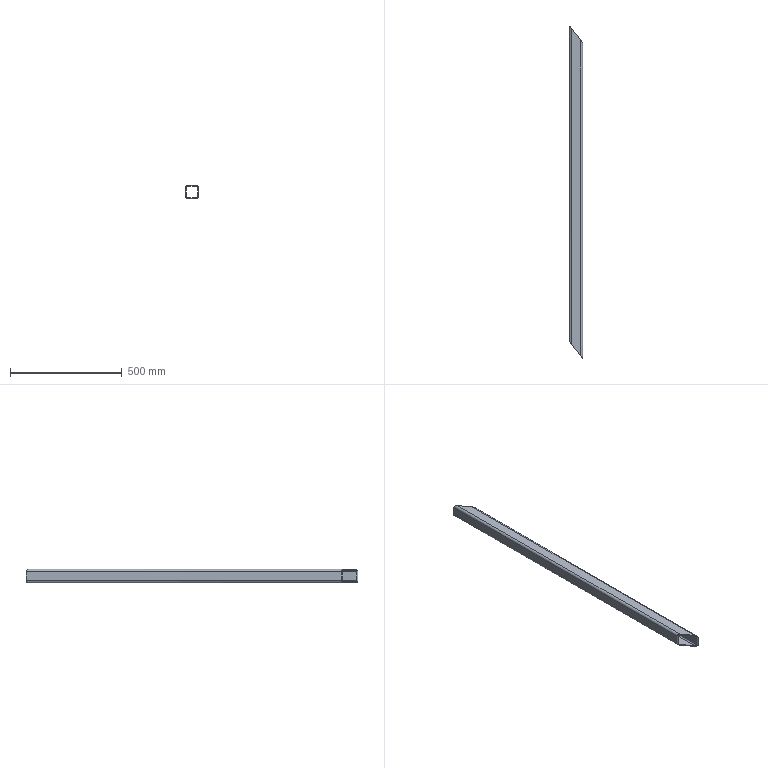Part | SolidWorks | features Extrusion 1, ICE 1 | 1 solid | 18 faces | box 60 x 1484 x 60 mm | volume 1185056 mm3 | plane 10 | cylinder 8 | commonest cylinder face diameters 12 x4 20 x4
STEP:
#1=CARTESIAN_POINT('',(-26.,70.025,-20.));
#2=VERTEX_POINT('',#1);
#3=CARTESIAN_POINT('',(-26.,70.025,20.));
#4=VERTEX_POINT('',#3);
#5=CARTESIAN_POINT('',(-26.,70.025,20.));
#6=DIRECTION('',(0.,0.,1.));
#7=VECTOR('',#6,1000.);
#8=LINE('',#5,#7);
#9=EDGE_CURVE('',#2,#4,#8,.T.);
#10=ORIENTED_EDGE('',*,*,#9,.F.);
#11=CARTESIAN_POINT('',(-26.,1479.025,-20.));
#12=VERTEX_POINT('',#11);
#13=CARTESIAN_POINT('',(-26.,2000.,-20.));
#14=DIRECTION('',(0.,-1.,0.));
#15=VECTOR('',#14,1000.);
#16=LINE('',#13,#15);
#17=EDGE_CURVE('',#12,#2,#16,.T.);
#18=ORIENTED_EDGE('',*,*,#17,.F.);
#19=CARTESIAN_POINT('',(-26.,1479.025,20.));
#20=VERTEX_POINT('',#19);
#21=CARTESIAN_POINT('',(-26.,1479.025,20.));
#22=DIRECTION('',(0.,0.,-1.));
#23=VECTOR('',#22,1000.);
#24=LINE('',#21,#23);
#25=EDGE_CURVE('',#20,#12,#24,.T.);
#26=ORIENTED_EDGE('',*,*,#25,.F.);
#27=CARTESIAN_POINT('',(-26.,2000.,20.));
#28=DIRECTION('',(0.,-1.,0.));
#29=VECTOR('',#28,1000.);
#30=LINE('',#27,#29);
#31=EDGE_CURVE('',#20,#4,#30,.T.);
#32=ORIENTED_EDGE('',*,*,#31,.T.);
#33=EDGE_LOOP('',(#10,#18,#26,#32));
#34=FACE_OUTER_BOUND('',#33,.T.);
#35=CARTESIAN_POINT('',(-26.,2000.,20.));
#36=DIRECTION('',(1.,0.,0.));
#37=DIRECTION('',(0.,0.,-1.));
#38=AXIS2_PLACEMENT_3D('',#35,#36,#37);
#39=PLANE('',#38);
#40=ADVANCED_FACE('',(#34),#39,.T.);
#41=CARTESIAN_POINT('',(-20.,62.523,-26.));
#42=VERTEX_POINT('',#41);
#43=CARTESIAN_POINT('',(-20.,62.523,-26.));
#44=CARTESIAN_POINT('',(-23.515,66.918,-26.));
#45=CARTESIAN_POINT('',(-26.,70.025,-23.515));
#46=CARTESIAN_POINT('',(-26.,70.025,-20.));
#47=(BOUNDED_CURVE()B_SPLINE_CURVE(3,(#43,#44,#45,#46),.UNSPECIFIED.,.F.,.T.)B_SPLINE_CURVE_WITH_KNOTS((4,4),(1.571,3.142),.UNSPECIFIED.)CURVE()GEOMETRIC_REPRESENTATION_ITEM()RATIONAL_B_SPLINE_CURVE((1.,0.8047,0.8047,1.))REPRESENTATION_ITEM(''));
#48=EDGE_CURVE('',#42,#2,#47,.T.);
#49=ORIENTED_EDGE('',*,*,#48,.F.);
#50=CARTESIAN_POINT('',(-20.,1471.523,-26.));
#51=VERTEX_POINT('',#50);
#52=CARTESIAN_POINT('',(-20.,2000.,-26.));
#53=DIRECTION('',(0.,-1.,0.));
#54=VECTOR('',#53,1000.);
#55=LINE('',#52,#54);
#56=EDGE_CURVE('',#51,#42,#55,.T.);
#57=ORIENTED_EDGE('',*,*,#56,.F.);
#58=CARTESIAN_POINT('',(-26.,1479.025,-20.));
#59=CARTESIAN_POINT('',(-26.,1479.025,-23.515));
#60=CARTESIAN_POINT('',(-23.515,1475.918,-26.));
#61=CARTESIAN_POINT('',(-20.,1471.523,-26.));
#62=(BOUNDED_CURVE()B_SPLINE_CURVE(3,(#58,#59,#60,#61),.UNSPECIFIED.,.F.,.F.)B_SPLINE_CURVE_WITH_KNOTS((4,4),(3.142,4.712),.UNSPECIFIED.)CURVE()GEOMETRIC_REPRESENTATION_ITEM()RATIONAL_B_SPLINE_CURVE((1.,0.8047,0.8047,1.))REPRESENTATION_ITEM(''));
#63=EDGE_CURVE('',#12,#51,#62,.T.);
#64=ORIENTED_EDGE('',*,*,#63,.F.);
#65=ORIENTED_EDGE('',*,*,#17,.T.);
#66=EDGE_LOOP('',(#49,#57,#64,#65));
#67=FACE_OUTER_BOUND('',#66,.T.);
#68=CARTESIAN_POINT('',(-20.,2000.,-20.));
#69=DIRECTION('',(0.,-1.,0.));
#70=DIRECTION('',(0.,0.,-1.));
#71=AXIS2_PLACEMENT_3D('',#68,#69,#70);
#72=CYLINDRICAL_SURFACE('',#71,6.);
#73=ADVANCED_FACE('',(#67),#72,.F.);
#74=CARTESIAN_POINT('',(20.,12.505,-26.));
#75=VERTEX_POINT('',#74);
#76=CARTESIAN_POINT('',(-965.035,1244.247,-26.));
#77=DIRECTION('',(-0.6246,0.781,0.));
#78=VECTOR('',#77,1000.);
#79=LINE('',#76,#78);
#80=EDGE_CURVE('',#75,#42,#79,.T.);
#81=ORIENTED_EDGE('',*,*,#80,.F.);
#82=CARTESIAN_POINT('',(20.,1421.505,-26.));
#83=VERTEX_POINT('',#82);
#84=CARTESIAN_POINT('',(20.,2000.,-26.));
#85=DIRECTION('',(0.,-1.,0.));
#86=VECTOR('',#85,1000.);
#87=LINE('',#84,#86);
#88=EDGE_CURVE('',#83,#75,#87,.T.);
#89=ORIENTED_EDGE('',*,*,#88,.F.);
#90=CARTESIAN_POINT('',(-277.773,1793.856,-26.));
#91=DIRECTION('',(0.6246,-0.781,0.));
#92=VECTOR('',#91,1000.);
#93=LINE('',#90,#92);
#94=EDGE_CURVE('',#51,#83,#93,.T.);
#95=ORIENTED_EDGE('',*,*,#94,.F.);
#96=ORIENTED_EDGE('',*,*,#56,.T.);
#97=EDGE_LOOP('',(#81,#89,#95,#96));
#98=FACE_OUTER_BOUND('',#97,.T.);
#99=CARTESIAN_POINT('',(-20.,2000.,-26.));
#100=DIRECTION('',(0.,0.,1.));
#101=DIRECTION('',(1.,0.,0.));
#102=AXIS2_PLACEMENT_3D('',#99,#100,#101);
#103=PLANE('',#102);
#104=ADVANCED_FACE('',(#98),#103,.T.);
#105=CARTESIAN_POINT('',(26.,5.002,-20.));
#106=VERTEX_POINT('',#105);
#107=CARTESIAN_POINT('',(26.,5.002,-20.));
#108=CARTESIAN_POINT('',(26.,5.002,-23.515));
#109=CARTESIAN_POINT('',(23.515,8.11,-26.));
#110=CARTESIAN_POINT('',(20.,12.505,-26.));
#111=(BOUNDED_CURVE()B_SPLINE_CURVE(3,(#107,#108,#109,#110),.UNSPECIFIED.,.F.,.F.)B_SPLINE_CURVE_WITH_KNOTS((4,4),(0.,1.571),.UNSPECIFIED.)CURVE()GEOMETRIC_REPRESENTATION_ITEM()RATIONAL_B_SPLINE_CURVE((1.,0.8047,0.8047,1.))REPRESENTATION_ITEM(''));
#112=EDGE_CURVE('',#106,#75,#111,.T.);
#113=ORIENTED_EDGE('',*,*,#112,.F.);
#114=CARTESIAN_POINT('',(26.,1414.002,-20.));
#115=VERTEX_POINT('',#114);
#116=CARTESIAN_POINT('',(26.,2000.,-20.));
#117=DIRECTION('',(0.,-1.,0.));
#118=VECTOR('',#117,1000.);
#119=LINE('',#116,#118);
#120=EDGE_CURVE('',#115,#106,#119,.T.);
#121=ORIENTED_EDGE('',*,*,#120,.F.);
#122=CARTESIAN_POINT('',(20.,1421.505,-26.));
#123=CARTESIAN_POINT('',(23.515,1417.11,-26.));
#124=CARTESIAN_POINT('',(26.,1414.002,-23.515));
#125=CARTESIAN_POINT('',(26.,1414.002,-20.));
#126=(BOUNDED_CURVE()B_SPLINE_CURVE(3,(#122,#123,#124,#125),.UNSPECIFIED.,.F.,.T.)B_SPLINE_CURVE_WITH_KNOTS((4,4),(4.712,6.283),.UNSPECIFIED.)CURVE()GEOMETRIC_REPRESENTATION_ITEM()RATIONAL_B_SPLINE_CURVE((1.,0.8047,0.8047,1.))REPRESENTATION_ITEM(''));
#127=EDGE_CURVE('',#83,#115,#126,.T.);
#128=ORIENTED_EDGE('',*,*,#127,.F.);
#129=ORIENTED_EDGE('',*,*,#88,.T.);
#130=EDGE_LOOP('',(#113,#121,#128,#129));
#131=FACE_OUTER_BOUND('',#130,.T.);
#132=CARTESIAN_POINT('',(20.,2000.,-20.));
#133=DIRECTION('',(0.,-1.,0.));
#134=DIRECTION('',(0.,0.,-1.));
#135=AXIS2_PLACEMENT_3D('',#132,#133,#134);
#136=CYLINDRICAL_SURFACE('',#135,6.);
#137=ADVANCED_FACE('',(#131),#136,.F.);
#138=CARTESIAN_POINT('',(26.,5.002,20.));
#139=VERTEX_POINT('',#138);
#140=CARTESIAN_POINT('',(26.,5.002,20.));
#141=DIRECTION('',(0.,0.,-1.));
#142=VECTOR('',#141,1000.);
#143=LINE('',#140,#142);
#144=EDGE_CURVE('',#139,#106,#143,.T.);
#145=ORIENTED_EDGE('',*,*,#144,.F.);
#146=CARTESIAN_POINT('',(26.,1414.002,20.));
#147=VERTEX_POINT('',#146);
#148=CARTESIAN_POINT('',(26.,2000.,20.));
#149=DIRECTION('',(0.,-1.,0.));
#150=VECTOR('',#149,1000.);
#151=LINE('',#148,#150);
#152=EDGE_CURVE('',#147,#139,#151,.T.);
#153=ORIENTED_EDGE('',*,*,#152,.F.);
#154=CARTESIAN_POINT('',(26.,1414.002,20.));
#155=DIRECTION('',(0.,0.,1.));
#156=VECTOR('',#155,1000.);
#157=LINE('',#154,#156);
#158=EDGE_CURVE('',#115,#147,#157,.T.);
#159=ORIENTED_EDGE('',*,*,#158,.F.);
#160=ORIENTED_EDGE('',*,*,#120,.T.);
#161=EDGE_LOOP('',(#145,#153,#159,#160));
#162=FACE_OUTER_BOUND('',#161,.T.);
#163=CARTESIAN_POINT('',(26.,2000.,20.));
#164=DIRECTION('',(-1.,0.,0.));
#165=DIRECTION('',(0.,0.,1.));
#166=AXIS2_PLACEMENT_3D('',#163,#164,#165);
#167=PLANE('',#166);
#168=ADVANCED_FACE('',(#162),#167,.T.);
#169=CARTESIAN_POINT('',(20.,12.505,26.));
#170=VERTEX_POINT('',#169);
#171=CARTESIAN_POINT('',(20.,12.505,26.));
#172=CARTESIAN_POINT('',(23.515,8.11,26.));
#173=CARTESIAN_POINT('',(26.,5.002,23.515));
#174=CARTESIAN_POINT('',(26.,5.002,20.));
#175=(BOUNDED_CURVE()B_SPLINE_CURVE(3,(#171,#172,#173,#174),.UNSPECIFIED.,.F.,.F.)B_SPLINE_CURVE_WITH_KNOTS((4,4),(4.712,6.283),.UNSPECIFIED.)CURVE()GEOMETRIC_REPRESENTATION_ITEM()RATIONAL_B_SPLINE_CURVE((1.,0.8047,0.8047,1.))REPRESENTATION_ITEM(''));
#176=EDGE_CURVE('',#170,#139,#175,.T.);
#177=ORIENTED_EDGE('',*,*,#176,.F.);
#178=CARTESIAN_POINT('',(20.,1421.505,26.));
#179=VERTEX_POINT('',#178);
#180=CARTESIAN_POINT('',(20.,2000.,26.));
#181=DIRECTION('',(0.,-1.,0.));
#182=VECTOR('',#181,1000.);
#183=LINE('',#180,#182);
#184=EDGE_CURVE('',#179,#170,#183,.T.);
#185=ORIENTED_EDGE('',*,*,#184,.F.);
#186=CARTESIAN_POINT('',(26.,1414.002,20.));
#187=CARTESIAN_POINT('',(26.,1414.002,23.515));
#188=CARTESIAN_POINT('',(23.515,1417.11,26.));
#189=CARTESIAN_POINT('',(20.,1421.505,26.));
#190=(BOUNDED_CURVE()B_SPLINE_CURVE(3,(#186,#187,#188,#189),.UNSPECIFIED.,.F.,.T.)B_SPLINE_CURVE_WITH_KNOTS((4,4),(0.,1.571),.UNSPECIFIED.)CURVE()GEOMETRIC_REPRESENTATION_ITEM()RATIONAL_B_SPLINE_CURVE((1.,0.8047,0.8047,1.))REPRESENTATION_ITEM(''));
#191=EDGE_CURVE('',#147,#179,#190,.T.);
#192=ORIENTED_EDGE('',*,*,#191,.F.);
#193=ORIENTED_EDGE('',*,*,#152,.T.);
#194=EDGE_LOOP('',(#177,#185,#192,#193));
#195=FACE_OUTER_BOUND('',#194,.T.);
#196=CARTESIAN_POINT('',(20.,2000.,20.));
#197=DIRECTION('',(0.,-1.,0.));
#198=DIRECTION('',(0.,0.,-1.));
#199=AXIS2_PLACEMENT_3D('',#196,#197,#198);
#200=CYLINDRICAL_SURFACE('',#199,6.);
#201=ADVANCED_FACE('',(#195),#200,.F.);
#202=CARTESIAN_POINT('',(-20.,62.523,26.));
#203=VERTEX_POINT('',#202);
#204=CARTESIAN_POINT('',(-965.035,1244.247,26.));
#205=DIRECTION('',(0.6246,-0.781,0.));
#206=VECTOR('',#205,1000.);
#207=LINE('',#204,#206);
#208=EDGE_CURVE('',#203,#170,#207,.T.);
#209=ORIENTED_EDGE('',*,*,#208,.F.);
#210=CARTESIAN_POINT('',(-20.,1471.523,26.));
#211=VERTEX_POINT('',#210);
#212=CARTESIAN_POINT('',(-20.,2000.,26.));
#213=DIRECTION('',(0.,-1.,0.));
#214=VECTOR('',#213,1000.);
#215=LINE('',#212,#214);
#216=EDGE_CURVE('',#211,#203,#215,.T.);
#217=ORIENTED_EDGE('',*,*,#216,.F.);
#218=CARTESIAN_POINT('',(-277.773,1793.856,26.));
#219=DIRECTION('',(-0.6246,0.781,0.));
#220=VECTOR('',#219,1000.);
#221=LINE('',#218,#220);
#222=EDGE_CURVE('',#179,#211,#221,.T.);
#223=ORIENTED_EDGE('',*,*,#222,.F.);
#224=ORIENTED_EDGE('',*,*,#184,.T.);
#225=EDGE_LOOP('',(#209,#217,#223,#224));
#226=FACE_OUTER_BOUND('',#225,.T.);
#227=CARTESIAN_POINT('',(-20.,2000.,26.));
#228=DIRECTION('',(0.,0.,-1.));
#229=DIRECTION('',(-1.,0.,0.));
#230=AXIS2_PLACEMENT_3D('',#227,#228,#229);
#231=PLANE('',#230);
#232=ADVANCED_FACE('',(#226),#231,.T.);
#233=CARTESIAN_POINT('',(-26.,70.025,20.));
#234=CARTESIAN_POINT('',(-26.,70.025,23.515));
#235=CARTESIAN_POINT('',(-23.515,66.918,26.));
#236=CARTESIAN_POINT('',(-20.,62.523,26.));
#237=(BOUNDED_CURVE()B_SPLINE_CURVE(3,(#233,#234,#235,#236),.UNSPECIFIED.,.F.,.F.)B_SPLINE_CURVE_WITH_KNOTS((4,4),(3.142,4.712),.UNSPECIFIED.)CURVE()GEOMETRIC_REPRESENTATION_ITEM()RATIONAL_B_SPLINE_CURVE((1.,0.8047,0.8047,1.))REPRESENTATION_ITEM(''));
#238=EDGE_CURVE('',#4,#203,#237,.T.);
#239=ORIENTED_EDGE('',*,*,#238,.F.);
#240=ORIENTED_EDGE('',*,*,#31,.F.);
#241=CARTESIAN_POINT('',(-20.,1471.523,26.));
#242=CARTESIAN_POINT('',(-23.515,1475.918,26.));
#243=CARTESIAN_POINT('',(-26.,1479.025,23.515));
#244=CARTESIAN_POINT('',(-26.,1479.025,20.));
#245=(BOUNDED_CURVE()B_SPLINE_CURVE(3,(#241,#242,#243,#244),.UNSPECIFIED.,.F.,.T.)B_SPLINE_CURVE_WITH_KNOTS((4,4),(1.571,3.142),.UNSPECIFIED.)CURVE()GEOMETRIC_REPRESENTATION_ITEM()RATIONAL_B_SPLINE_CURVE((1.,0.8047,0.8047,1.))REPRESENTATION_ITEM(''));
#246=EDGE_CURVE('',#211,#20,#245,.T.);
#247=ORIENTED_EDGE('',*,*,#246,.F.);
#248=ORIENTED_EDGE('',*,*,#216,.T.);
#249=EDGE_LOOP('',(#239,#240,#247,#248));
#250=FACE_OUTER_BOUND('',#249,.T.);
#251=CARTESIAN_POINT('',(-20.,2000.,20.));
#252=DIRECTION('',(0.,-1.,0.));
#253=DIRECTION('',(0.,0.,-1.));
#254=AXIS2_PLACEMENT_3D('',#251,#252,#253);
#255=CYLINDRICAL_SURFACE('',#254,6.);
#256=ADVANCED_FACE('',(#250),#255,.F.);
#257=ORIENTED_EDGE('',*,*,#246,.T.);
#258=ORIENTED_EDGE('',*,*,#25,.T.);
#259=ORIENTED_EDGE('',*,*,#63,.T.);
#260=ORIENTED_EDGE('',*,*,#94,.T.);
#261=ORIENTED_EDGE('',*,*,#127,.T.);
#262=ORIENTED_EDGE('',*,*,#158,.T.);
#263=ORIENTED_EDGE('',*,*,#191,.T.);
#264=ORIENTED_EDGE('',*,*,#222,.T.);
#265=EDGE_LOOP('',(#257,#258,#259,#260,#261,#262,#263,#264));
#266=FACE_BOUND('',#265,.T.);
#267=CARTESIAN_POINT('',(-20.,1471.523,-30.));
#268=VERTEX_POINT('',#267);
#269=CARTESIAN_POINT('',(20.,1421.505,-30.));
#270=VERTEX_POINT('',#269);
#271=CARTESIAN_POINT('',(-30.,1484.027,-30.));
#272=DIRECTION('',(0.6246,-0.781,0.));
#273=VECTOR('',#272,1000.);
#274=LINE('',#271,#273);
#275=EDGE_CURVE('',#268,#270,#274,.T.);
#276=ORIENTED_EDGE('',*,*,#275,.F.);
#277=CARTESIAN_POINT('',(-30.,1484.027,-20.));
#278=VERTEX_POINT('',#277);
#279=CARTESIAN_POINT('',(-30.,1484.027,-20.));
#280=CARTESIAN_POINT('',(-30.,1484.027,-25.858));
#281=CARTESIAN_POINT('',(-25.858,1478.848,-30.));
#282=CARTESIAN_POINT('',(-20.,1471.523,-30.));
#283=(BOUNDED_CURVE()B_SPLINE_CURVE(3,(#279,#280,#281,#282),.UNSPECIFIED.,.F.,.F.)B_SPLINE_CURVE_WITH_KNOTS((4,4),(3.142,4.712),.UNSPECIFIED.)CURVE()GEOMETRIC_REPRESENTATION_ITEM()RATIONAL_B_SPLINE_CURVE((1.,0.8047,0.8047,1.))REPRESENTATION_ITEM(''));
#284=EDGE_CURVE('',#278,#268,#283,.T.);
#285=ORIENTED_EDGE('',*,*,#284,.F.);
#286=CARTESIAN_POINT('',(-30.,1484.027,20.));
#287=VERTEX_POINT('',#286);
#288=CARTESIAN_POINT('',(-30.,1484.027,-30.));
#289=DIRECTION('',(0.,0.,1.));
#290=VECTOR('',#289,1000.);
#291=LINE('',#288,#290);
#292=EDGE_CURVE('',#278,#287,#291,.T.);
#293=ORIENTED_EDGE('',*,*,#292,.T.);
#294=CARTESIAN_POINT('',(-20.,1471.523,30.));
#295=VERTEX_POINT('',#294);
#296=CARTESIAN_POINT('',(-20.,1471.523,30.));
#297=CARTESIAN_POINT('',(-25.858,1478.848,30.));
#298=CARTESIAN_POINT('',(-30.,1484.027,25.858));
#299=CARTESIAN_POINT('',(-30.,1484.027,20.));
#300=(BOUNDED_CURVE()B_SPLINE_CURVE(3,(#296,#297,#298,#299),.UNSPECIFIED.,.F.,.T.)B_SPLINE_CURVE_WITH_KNOTS((4,4),(1.571,3.142),.UNSPECIFIED.)CURVE()GEOMETRIC_REPRESENTATION_ITEM()RATIONAL_B_SPLINE_CURVE((1.,0.8047,0.8047,1.))REPRESENTATION_ITEM(''));
#301=EDGE_CURVE('',#295,#287,#300,.T.);
#302=ORIENTED_EDGE('',*,*,#301,.F.);
#303=CARTESIAN_POINT('',(20.,1421.505,30.));
#304=VERTEX_POINT('',#303);
#305=CARTESIAN_POINT('',(-277.773,1793.856,30.));
#306=DIRECTION('',(-0.6246,0.781,0.));
#307=VECTOR('',#306,1000.);
#308=LINE('',#305,#307);
#309=EDGE_CURVE('',#304,#295,#308,.T.);
#310=ORIENTED_EDGE('',*,*,#309,.F.);
#311=CARTESIAN_POINT('',(30.,1409.,20.));
#312=VERTEX_POINT('',#311);
#313=CARTESIAN_POINT('',(30.,1409.,20.));
#314=CARTESIAN_POINT('',(30.,1409.,25.858));
#315=CARTESIAN_POINT('',(25.858,1414.18,30.));
#316=CARTESIAN_POINT('',(20.,1421.505,30.));
#317=(BOUNDED_CURVE()B_SPLINE_CURVE(3,(#313,#314,#315,#316),.UNSPECIFIED.,.F.,.F.)B_SPLINE_CURVE_WITH_KNOTS((4,4),(0.,1.571),.UNSPECIFIED.)CURVE()GEOMETRIC_REPRESENTATION_ITEM()RATIONAL_B_SPLINE_CURVE((1.,0.8047,0.8047,1.))REPRESENTATION_ITEM(''));
#318=EDGE_CURVE('',#312,#304,#317,.T.);
#319=ORIENTED_EDGE('',*,*,#318,.F.);
#320=CARTESIAN_POINT('',(30.,1409.,-20.));
#321=VERTEX_POINT('',#320);
#322=CARTESIAN_POINT('',(30.,1409.,-30.));
#323=DIRECTION('',(0.,0.,1.));
#324=VECTOR('',#323,1000.);
#325=LINE('',#322,#324);
#326=EDGE_CURVE('',#321,#312,#325,.T.);
#327=ORIENTED_EDGE('',*,*,#326,.F.);
#328=CARTESIAN_POINT('',(20.,1421.505,-30.));
#329=CARTESIAN_POINT('',(25.858,1414.18,-30.));
#330=CARTESIAN_POINT('',(30.,1409.,-25.858));
#331=CARTESIAN_POINT('',(30.,1409.,-20.));
#332=(BOUNDED_CURVE()B_SPLINE_CURVE(3,(#328,#329,#330,#331),.UNSPECIFIED.,.F.,.F.)B_SPLINE_CURVE_WITH_KNOTS((4,4),(4.712,6.283),.UNSPECIFIED.)CURVE()GEOMETRIC_REPRESENTATION_ITEM()RATIONAL_B_SPLINE_CURVE((1.,0.8047,0.8047,1.))REPRESENTATION_ITEM(''));
#333=EDGE_CURVE('',#270,#321,#332,.T.);
#334=ORIENTED_EDGE('',*,*,#333,.F.);
#335=EDGE_LOOP('',(#276,#285,#293,#302,#310,#319,#327,#334));
#336=FACE_OUTER_BOUND('',#335,.T.);
#337=CARTESIAN_POINT('',(-30.,1484.027,-30.));
#338=DIRECTION('',(-0.781,-0.6246,0.));
#339=DIRECTION('',(0.6246,-0.781,0.));
#340=AXIS2_PLACEMENT_3D('',#337,#338,#339);
#341=PLANE('',#340);
#342=ADVANCED_FACE('',(#266,#336),#341,.F.);
#343=ORIENTED_EDGE('',*,*,#238,.T.);
#344=ORIENTED_EDGE('',*,*,#208,.T.);
#345=ORIENTED_EDGE('',*,*,#176,.T.);
#346=ORIENTED_EDGE('',*,*,#144,.T.);
#347=ORIENTED_EDGE('',*,*,#112,.T.);
#348=ORIENTED_EDGE('',*,*,#80,.T.);
#349=ORIENTED_EDGE('',*,*,#48,.T.);
#350=ORIENTED_EDGE('',*,*,#9,.T.);
#351=EDGE_LOOP('',(#343,#344,#345,#346,#347,#348,#349,#350));
#352=FACE_BOUND('',#351,.T.);
#353=CARTESIAN_POINT('',(30.,0.,20.));
#354=VERTEX_POINT('',#353);
#355=CARTESIAN_POINT('',(30.,0.,-20.));
#356=VERTEX_POINT('',#355);
#357=CARTESIAN_POINT('',(30.,0.,20.));
#358=DIRECTION('',(0.,0.,-1.));
#359=VECTOR('',#358,1000.);
#360=LINE('',#357,#359);
#361=EDGE_CURVE('',#354,#356,#360,.T.);
#362=ORIENTED_EDGE('',*,*,#361,.F.);
#363=CARTESIAN_POINT('',(20.,12.505,30.));
#364=VERTEX_POINT('',#363);
#365=CARTESIAN_POINT('',(20.,12.505,30.));
#366=CARTESIAN_POINT('',(25.858,5.18,30.));
#367=CARTESIAN_POINT('',(30.,0.,25.858));
#368=CARTESIAN_POINT('',(30.,0.,20.));
#369=(BOUNDED_CURVE()B_SPLINE_CURVE(3,(#365,#366,#367,#368),.UNSPECIFIED.,.F.,.T.)B_SPLINE_CURVE_WITH_KNOTS((4,4),(4.712,6.283),.UNSPECIFIED.)CURVE()GEOMETRIC_REPRESENTATION_ITEM()RATIONAL_B_SPLINE_CURVE((1.,0.8047,0.8047,1.))REPRESENTATION_ITEM(''));
#370=EDGE_CURVE('',#364,#354,#369,.T.);
#371=ORIENTED_EDGE('',*,*,#370,.F.);
#372=CARTESIAN_POINT('',(-20.,62.523,30.));
#373=VERTEX_POINT('',#372);
#374=CARTESIAN_POINT('',(-965.035,1244.247,30.));
#375=DIRECTION('',(0.6246,-0.781,0.));
#376=VECTOR('',#375,1000.);
#377=LINE('',#374,#376);
#378=EDGE_CURVE('',#373,#364,#377,.T.);
#379=ORIENTED_EDGE('',*,*,#378,.F.);
#380=CARTESIAN_POINT('',(-30.,75.027,20.));
#381=VERTEX_POINT('',#380);
#382=CARTESIAN_POINT('',(-30.,75.027,20.));
#383=CARTESIAN_POINT('',(-30.,75.027,25.858));
#384=CARTESIAN_POINT('',(-25.858,69.848,30.));
#385=CARTESIAN_POINT('',(-20.,62.523,30.));
#386=(BOUNDED_CURVE()B_SPLINE_CURVE(3,(#382,#383,#384,#385),.UNSPECIFIED.,.F.,.T.)B_SPLINE_CURVE_WITH_KNOTS((4,4),(3.142,4.712),.UNSPECIFIED.)CURVE()GEOMETRIC_REPRESENTATION_ITEM()RATIONAL_B_SPLINE_CURVE((1.,0.8047,0.8047,1.))REPRESENTATION_ITEM(''));
#387=EDGE_CURVE('',#381,#373,#386,.T.);
#388=ORIENTED_EDGE('',*,*,#387,.F.);
#389=CARTESIAN_POINT('',(-30.,75.027,-20.));
#390=VERTEX_POINT('',#389);
#391=CARTESIAN_POINT('',(-30.,75.027,-30.));
#392=DIRECTION('',(0.,0.,1.));
#393=VECTOR('',#392,1000.);
#394=LINE('',#391,#393);
#395=EDGE_CURVE('',#390,#381,#394,.T.);
#396=ORIENTED_EDGE('',*,*,#395,.F.);
#397=CARTESIAN_POINT('',(-20.,62.523,-30.));
#398=VERTEX_POINT('',#397);
#399=CARTESIAN_POINT('',(-20.,62.523,-30.));
#400=CARTESIAN_POINT('',(-25.858,69.848,-30.));
#401=CARTESIAN_POINT('',(-30.,75.027,-25.858));
#402=CARTESIAN_POINT('',(-30.,75.027,-20.));
#403=(BOUNDED_CURVE()B_SPLINE_CURVE(3,(#399,#400,#401,#402),.UNSPECIFIED.,.F.,.F.)B_SPLINE_CURVE_WITH_KNOTS((4,4),(1.571,3.142),.UNSPECIFIED.)CURVE()GEOMETRIC_REPRESENTATION_ITEM()RATIONAL_B_SPLINE_CURVE((1.,0.8047,0.8047,1.))REPRESENTATION_ITEM(''));
#404=EDGE_CURVE('',#398,#390,#403,.T.);
#405=ORIENTED_EDGE('',*,*,#404,.F.);
#406=CARTESIAN_POINT('',(20.,12.505,-30.));
#407=VERTEX_POINT('',#406);
#408=CARTESIAN_POINT('',(30.,0.,-30.));
#409=DIRECTION('',(-0.6246,0.781,0.));
#410=VECTOR('',#409,1000.);
#411=LINE('',#408,#410);
#412=EDGE_CURVE('',#407,#398,#411,.T.);
#413=ORIENTED_EDGE('',*,*,#412,.F.);
#414=CARTESIAN_POINT('',(30.,0.,-20.));
#415=CARTESIAN_POINT('',(30.,0.,-25.858));
#416=CARTESIAN_POINT('',(25.858,5.18,-30.));
#417=CARTESIAN_POINT('',(20.,12.505,-30.));
#418=(BOUNDED_CURVE()B_SPLINE_CURVE(3,(#414,#415,#416,#417),.UNSPECIFIED.,.F.,.T.)B_SPLINE_CURVE_WITH_KNOTS((4,4),(0.,1.571),.UNSPECIFIED.)CURVE()GEOMETRIC_REPRESENTATION_ITEM()RATIONAL_B_SPLINE_CURVE((1.,0.8047,0.8047,1.))REPRESENTATION_ITEM(''));
#419=EDGE_CURVE('',#356,#407,#418,.T.);
#420=ORIENTED_EDGE('',*,*,#419,.F.);
#421=EDGE_LOOP('',(#362,#371,#379,#388,#396,#405,#413,#420));
#422=FACE_OUTER_BOUND('',#421,.T.);
#423=CARTESIAN_POINT('',(30.,0.,-30.));
#424=DIRECTION('',(0.781,0.6246,0.));
#425=DIRECTION('',(-0.6246,0.781,0.));
#426=AXIS2_PLACEMENT_3D('',#423,#424,#425);
#427=PLANE('',#426);
#428=ADVANCED_FACE('',(#352,#422),#427,.F.);
#429=CARTESIAN_POINT('',(20.,2000.,30.));
#430=DIRECTION('',(0.,-1.,0.));
#431=VECTOR('',#430,1000.);
#432=LINE('',#429,#431);
#433=EDGE_CURVE('',#304,#364,#432,.T.);
#434=ORIENTED_EDGE('',*,*,#433,.T.);
#435=ORIENTED_EDGE('',*,*,#370,.T.);
#436=CARTESIAN_POINT('',(30.,2000.,20.));
#437=DIRECTION('',(0.,-1.,0.));
#438=VECTOR('',#437,1000.);
#439=LINE('',#436,#438);
#440=EDGE_CURVE('',#312,#354,#439,.T.);
#441=ORIENTED_EDGE('',*,*,#440,.F.);
#442=ORIENTED_EDGE('',*,*,#318,.T.);
#443=EDGE_LOOP('',(#434,#435,#441,#442));
#444=FACE_OUTER_BOUND('',#443,.T.);
#445=CARTESIAN_POINT('',(20.,2000.,20.));
#446=DIRECTION('',(0.,-1.,0.));
#447=DIRECTION('',(0.,0.,-1.));
#448=AXIS2_PLACEMENT_3D('',#445,#446,#447);
#449=CYLINDRICAL_SURFACE('',#448,10.);
#450=ADVANCED_FACE('',(#444),#449,.T.);
#451=CARTESIAN_POINT('',(30.,2000.,-20.));
#452=DIRECTION('',(0.,-1.,0.));
#453=VECTOR('',#452,1000.);
#454=LINE('',#451,#453);
#455=EDGE_CURVE('',#321,#356,#454,.T.);
#456=ORIENTED_EDGE('',*,*,#455,.F.);
#457=ORIENTED_EDGE('',*,*,#326,.T.);
#458=ORIENTED_EDGE('',*,*,#440,.T.);
#459=ORIENTED_EDGE('',*,*,#361,.T.);
#460=EDGE_LOOP('',(#456,#457,#458,#459));
#461=FACE_OUTER_BOUND('',#460,.T.);
#462=CARTESIAN_POINT('',(30.,2000.,20.));
#463=DIRECTION('',(-1.,0.,0.));
#464=DIRECTION('',(0.,0.,1.));
#465=AXIS2_PLACEMENT_3D('',#462,#463,#464);
#466=PLANE('',#465);
#467=ADVANCED_FACE('',(#461),#466,.F.);
#468=ORIENTED_EDGE('',*,*,#455,.T.);
#469=ORIENTED_EDGE('',*,*,#419,.T.);
#470=CARTESIAN_POINT('',(20.,2000.,-30.));
#471=DIRECTION('',(0.,-1.,0.));
#472=VECTOR('',#471,1000.);
#473=LINE('',#470,#472);
#474=EDGE_CURVE('',#270,#407,#473,.T.);
#475=ORIENTED_EDGE('',*,*,#474,.F.);
#476=ORIENTED_EDGE('',*,*,#333,.T.);
#477=EDGE_LOOP('',(#468,#469,#475,#476));
#478=FACE_OUTER_BOUND('',#477,.T.);
#479=CARTESIAN_POINT('',(20.,2000.,-20.));
#480=DIRECTION('',(0.,-1.,0.));
#481=DIRECTION('',(0.,0.,-1.));
#482=AXIS2_PLACEMENT_3D('',#479,#480,#481);
#483=CYLINDRICAL_SURFACE('',#482,10.);
#484=ADVANCED_FACE('',(#478),#483,.T.);
#485=ORIENTED_EDGE('',*,*,#474,.T.);
#486=ORIENTED_EDGE('',*,*,#412,.T.);
#487=CARTESIAN_POINT('',(-20.,2000.,-30.));
#488=DIRECTION('',(0.,-1.,0.));
#489=VECTOR('',#488,1000.);
#490=LINE('',#487,#489);
#491=EDGE_CURVE('',#268,#398,#490,.T.);
#492=ORIENTED_EDGE('',*,*,#491,.F.);
#493=ORIENTED_EDGE('',*,*,#275,.T.);
#494=EDGE_LOOP('',(#485,#486,#492,#493));
#495=FACE_OUTER_BOUND('',#494,.T.);
#496=CARTESIAN_POINT('',(-20.,2000.,-30.));
#497=DIRECTION('',(0.,0.,1.));
#498=DIRECTION('',(1.,0.,0.));
#499=AXIS2_PLACEMENT_3D('',#496,#497,#498);
#500=PLANE('',#499);
#501=ADVANCED_FACE('',(#495),#500,.F.);
#502=ORIENTED_EDGE('',*,*,#491,.T.);
#503=ORIENTED_EDGE('',*,*,#404,.T.);
#504=CARTESIAN_POINT('',(-30.,2000.,-20.));
#505=DIRECTION('',(0.,-1.,0.));
#506=VECTOR('',#505,1000.);
#507=LINE('',#504,#506);
#508=EDGE_CURVE('',#278,#390,#507,.T.);
#509=ORIENTED_EDGE('',*,*,#508,.F.);
#510=ORIENTED_EDGE('',*,*,#284,.T.);
#511=EDGE_LOOP('',(#502,#503,#509,#510));
#512=FACE_OUTER_BOUND('',#511,.T.);
#513=CARTESIAN_POINT('',(-20.,2000.,-20.));
#514=DIRECTION('',(0.,-1.,0.));
#515=DIRECTION('',(0.,0.,-1.));
#516=AXIS2_PLACEMENT_3D('',#513,#514,#515);
#517=CYLINDRICAL_SURFACE('',#516,10.);
#518=ADVANCED_FACE('',(#512),#517,.T.);
#519=ORIENTED_EDGE('',*,*,#508,.T.);
#520=ORIENTED_EDGE('',*,*,#395,.T.);
#521=CARTESIAN_POINT('',(-30.,2000.,20.));
#522=DIRECTION('',(0.,-1.,0.));
#523=VECTOR('',#522,1000.);
#524=LINE('',#521,#523);
#525=EDGE_CURVE('',#287,#381,#524,.T.);
#526=ORIENTED_EDGE('',*,*,#525,.F.);
#527=ORIENTED_EDGE('',*,*,#292,.F.);
#528=EDGE_LOOP('',(#519,#520,#526,#527));
#529=FACE_OUTER_BOUND('',#528,.T.);
#530=CARTESIAN_POINT('',(-30.,2000.,20.));
#531=DIRECTION('',(1.,0.,0.));
#532=DIRECTION('',(0.,0.,-1.));
#533=AXIS2_PLACEMENT_3D('',#530,#531,#532);
#534=PLANE('',#533);
#535=ADVANCED_FACE('',(#529),#534,.F.);
#536=ORIENTED_EDGE('',*,*,#525,.T.);
#537=ORIENTED_EDGE('',*,*,#387,.T.);
#538=CARTESIAN_POINT('',(-20.,2000.,30.));
#539=DIRECTION('',(0.,-1.,0.));
#540=VECTOR('',#539,1000.);
#541=LINE('',#538,#540);
#542=EDGE_CURVE('',#295,#373,#541,.T.);
#543=ORIENTED_EDGE('',*,*,#542,.F.);
#544=ORIENTED_EDGE('',*,*,#301,.T.);
#545=EDGE_LOOP('',(#536,#537,#543,#544));
#546=FACE_OUTER_BOUND('',#545,.T.);
#547=CARTESIAN_POINT('',(-20.,2000.,20.));
#548=DIRECTION('',(0.,-1.,0.));
#549=DIRECTION('',(0.,0.,-1.));
#550=AXIS2_PLACEMENT_3D('',#547,#548,#549);
#551=CYLINDRICAL_SURFACE('',#550,10.);
#552=ADVANCED_FACE('',(#546),#551,.T.);
#553=ORIENTED_EDGE('',*,*,#542,.T.);
#554=ORIENTED_EDGE('',*,*,#378,.T.);
#555=ORIENTED_EDGE('',*,*,#433,.F.);
#556=ORIENTED_EDGE('',*,*,#309,.T.);
#557=EDGE_LOOP('',(#553,#554,#555,#556));
#558=FACE_OUTER_BOUND('',#557,.T.);
#559=CARTESIAN_POINT('',(-20.,2000.,30.));
#560=DIRECTION('',(0.,0.,-1.));
#561=DIRECTION('',(-1.,0.,0.));
#562=AXIS2_PLACEMENT_3D('',#559,#560,#561);
#563=PLANE('',#562);
#564=ADVANCED_FACE('',(#558),#563,.F.);
#565=CLOSED_SHELL('',(#40,#73,#104,#137,#168,#201,#232,#256,#342,#428,#450,#467,#484,#501,#518,#535,#552,#564));
#566=MANIFOLD_SOLID_BREP('',#565);
#567=CARTESIAN_POINT('',(0.,0.,0.));
#568=DIRECTION('',(0.,0.,1.));
#569=DIRECTION('',(1.,0.,0.));
#570=AXIS2_PLACEMENT_3D('',#567,#568,#569);
#571=(LENGTH_UNIT()NAMED_UNIT(*)SI_UNIT(.MILLI.,.METRE.));
#572=UNCERTAINTY_MEASURE_WITH_UNIT(LENGTH_MEASURE(0.00001),#571,'','');
#573=(NAMED_UNIT(*)PLANE_ANGLE_UNIT()SI_UNIT($,.RADIAN.));
#574=(NAMED_UNIT(*)SI_UNIT($,.STERADIAN.)SOLID_ANGLE_UNIT());
#575=(GEOMETRIC_REPRESENTATION_CONTEXT(3)GLOBAL_UNCERTAINTY_ASSIGNED_CONTEXT((#572))GLOBAL_UNIT_ASSIGNED_CONTEXT((#571,#573,#574))REPRESENTATION_CONTEXT('',''));
#576=ADVANCED_BREP_SHAPE_REPRESENTATION('',(#566,#570),#575);